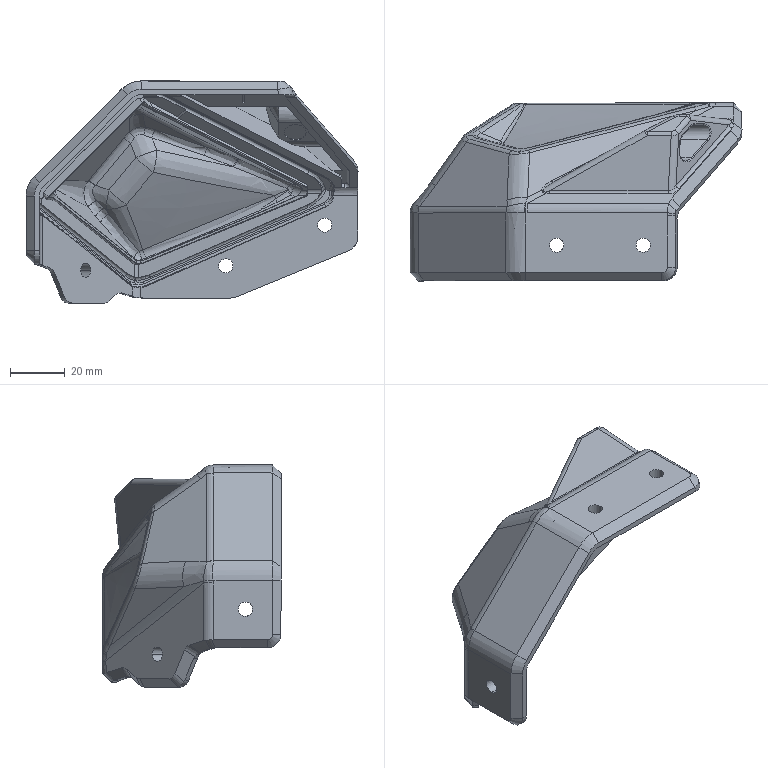Part | SolidWorks | features BaseBody 1 | 1 solid | 516 faces | box 121.217 x 65.032 x 81.078 mm | volume 61665 mm3 | spline 189 | cylinder 163 | plane 147 | sphere 6 | cone 6 | torus 5 | commonest cylinder face diameters 0.6 x18 4 x15 5.2 x15 0.4 x14 10 x13 8 x12